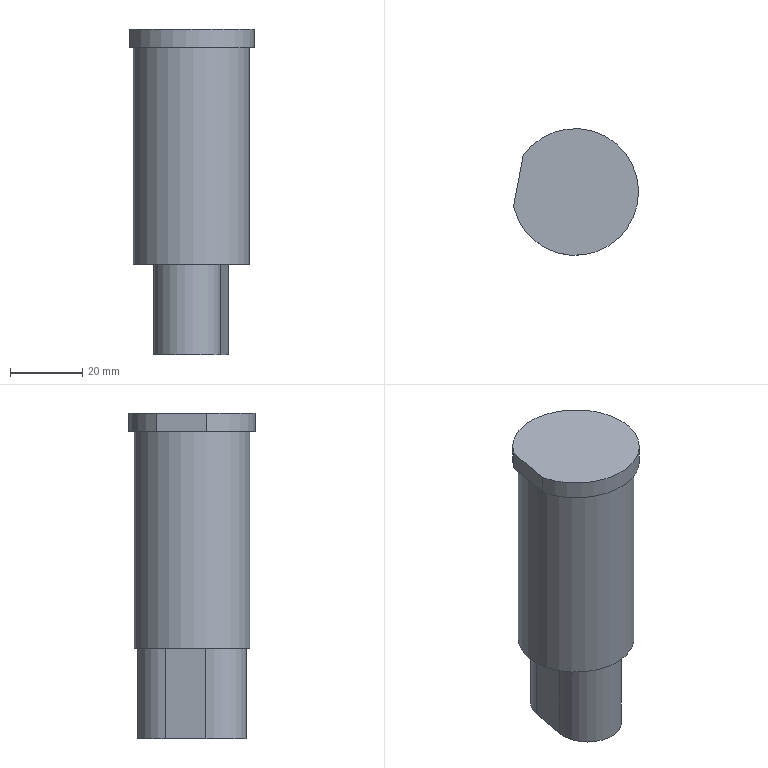Part | NX | features solid 2 | 1 solid | 11 faces | box 34.539 x 35 x 90 mm | volume 65190 mm3 | plane 7 | cylinder 4 | commonest cylinder face diameters 18.7 x2 32 x1 35 x1
STEP:
#1=CARTESIAN_POINT('',(-660.007,435.289,33.));
#2=VERTEX_POINT('',#1);
#3=CARTESIAN_POINT('',(-675.728,438.265,33.));
#4=DIRECTION('',(0.,0.,-1.));
#5=DIRECTION('',(0.9826,-0.186,0.));
#6=AXIS2_PLACEMENT_3D('',#3,#4,#5);
#7=CIRCLE('',#6,16.);
#8=EDGE_CURVE('',#2,#2,#7,.T.);
#9=ORIENTED_EDGE('',*,*,#8,.T.);
#10=EDGE_LOOP('',(#9));
#11=FACE_BOUND('',#10,.T.);
#12=CARTESIAN_POINT('',(-667.602,430.926,33.));
#13=VERTEX_POINT('',#12);
#14=CARTESIAN_POINT('',(-665.481,442.127,33.));
#15=VERTEX_POINT('',#14);
#16=CARTESIAN_POINT('',(-666.541,436.526,33.));
#17=DIRECTION('',(0.186,0.9826,0.));
#18=VECTOR('',#17,1000.);
#19=LINE('',#16,#18);
#20=EDGE_CURVE('',#13,#15,#19,.T.);
#21=ORIENTED_EDGE('',*,*,#20,.T.);
#22=CARTESIAN_POINT('',(-683.855,445.605,33.));
#23=VERTEX_POINT('',#22);
#24=CARTESIAN_POINT('',(-674.668,443.866,33.));
#25=DIRECTION('',(0.,0.,-1.));
#26=DIRECTION('',(0.9826,-0.186,0.));
#27=AXIS2_PLACEMENT_3D('',#24,#25,#26);
#28=CIRCLE('',#27,9.35);
#29=EDGE_CURVE('',#23,#15,#28,.T.);
#30=ORIENTED_EDGE('',*,*,#29,.F.);
#31=CARTESIAN_POINT('',(-685.975,434.403,33.));
#32=VERTEX_POINT('',#31);
#33=CARTESIAN_POINT('',(-684.915,440.004,33.));
#34=DIRECTION('',(0.186,0.9826,0.));
#35=VECTOR('',#34,1000.);
#36=LINE('',#33,#35);
#37=EDGE_CURVE('',#32,#23,#36,.T.);
#38=ORIENTED_EDGE('',*,*,#37,.F.);
#39=CARTESIAN_POINT('',(-676.788,432.665,33.));
#40=DIRECTION('',(0.,0.,-1.));
#41=DIRECTION('',(0.9826,-0.186,0.));
#42=AXIS2_PLACEMENT_3D('',#39,#40,#41);
#43=CIRCLE('',#42,9.35);
#44=EDGE_CURVE('',#13,#32,#43,.T.);
#45=ORIENTED_EDGE('',*,*,#44,.F.);
#46=EDGE_LOOP('',(#21,#30,#38,#45));
#47=FACE_BOUND('',#46,.T.);
#48=CARTESIAN_POINT('',(-675.728,438.265,33.));
#49=DIRECTION('',(0.,0.,1.));
#50=DIRECTION('',(0.9826,-0.186,0.));
#51=AXIS2_PLACEMENT_3D('',#48,#49,#50);
#52=PLANE('',#51);
#53=ADVANCED_FACE('',(#11,#47),#52,.F.);
#54=ORIENTED_EDGE('',*,*,#8,.F.);
#55=EDGE_LOOP('',(#54));
#56=FACE_BOUND('',#55,.T.);
#57=CARTESIAN_POINT('',(-691.449,441.241,93.));
#58=VERTEX_POINT('',#57);
#59=CARTESIAN_POINT('',(-675.728,438.265,93.));
#60=DIRECTION('',(0.,0.,-1.));
#61=DIRECTION('',(0.9826,-0.186,0.));
#62=AXIS2_PLACEMENT_3D('',#59,#60,#61);
#63=CIRCLE('',#62,16.);
#64=EDGE_CURVE('',#58,#58,#63,.T.);
#65=ORIENTED_EDGE('',*,*,#64,.T.);
#66=EDGE_LOOP('',(#65));
#67=FACE_BOUND('',#66,.T.);
#68=CARTESIAN_POINT('',(-675.728,438.265,98.));
#69=DIRECTION('',(0.,0.,-1.));
#70=DIRECTION('',(-0.9826,0.186,0.));
#71=AXIS2_PLACEMENT_3D('',#68,#69,#70);
#72=CYLINDRICAL_SURFACE('',#71,16.);
#73=ADVANCED_FACE('',(#56,#67),#72,.T.);
#74=CARTESIAN_POINT('',(-690.131,448.206,93.));
#75=VERTEX_POINT('',#74);
#76=CARTESIAN_POINT('',(-692.768,434.276,93.));
#77=VERTEX_POINT('',#76);
#78=CARTESIAN_POINT('',(-675.728,438.265,93.));
#79=DIRECTION('',(0.,0.,-1.));
#80=DIRECTION('',(0.9826,-0.186,0.));
#81=AXIS2_PLACEMENT_3D('',#78,#79,#80);
#82=CIRCLE('',#81,17.5);
#83=EDGE_CURVE('',#75,#77,#82,.T.);
#84=ORIENTED_EDGE('',*,*,#83,.T.);
#85=CARTESIAN_POINT('',(-691.449,441.241,93.));
#86=DIRECTION('',(-0.186,-0.9826,0.));
#87=VECTOR('',#86,1000.);
#88=LINE('',#85,#87);
#89=EDGE_CURVE('',#58,#77,#88,.T.);
#90=ORIENTED_EDGE('',*,*,#89,.F.);
#91=ORIENTED_EDGE('',*,*,#64,.F.);
#92=CARTESIAN_POINT('',(-691.449,441.241,93.));
#93=DIRECTION('',(-0.186,-0.9826,0.));
#94=VECTOR('',#93,1000.);
#95=LINE('',#92,#94);
#96=EDGE_CURVE('',#75,#58,#95,.T.);
#97=ORIENTED_EDGE('',*,*,#96,.F.);
#98=EDGE_LOOP('',(#84,#90,#91,#97));
#99=FACE_BOUND('',#98,.T.);
#100=CARTESIAN_POINT('',(-675.728,438.265,93.));
#101=DIRECTION('',(0.,0.,1.));
#102=DIRECTION('',(0.9826,-0.186,0.));
#103=AXIS2_PLACEMENT_3D('',#100,#101,#102);
#104=PLANE('',#103);
#105=ADVANCED_FACE('',(#99),#104,.F.);
#106=CARTESIAN_POINT('',(-692.768,434.276,98.));
#107=VERTEX_POINT('',#106);
#108=CARTESIAN_POINT('',(-692.768,434.276,102.));
#109=DIRECTION('',(0.,0.,-1.));
#110=VECTOR('',#109,1000.);
#111=LINE('',#108,#110);
#112=EDGE_CURVE('',#107,#77,#111,.T.);
#113=ORIENTED_EDGE('',*,*,#112,.T.);
#114=ORIENTED_EDGE('',*,*,#83,.F.);
#115=CARTESIAN_POINT('',(-690.131,448.206,98.));
#116=VERTEX_POINT('',#115);
#117=CARTESIAN_POINT('',(-690.131,448.206,102.));
#118=DIRECTION('',(0.,0.,-1.));
#119=VECTOR('',#118,1000.);
#120=LINE('',#117,#119);
#121=EDGE_CURVE('',#75,#116,#120,.F.);
#122=ORIENTED_EDGE('',*,*,#121,.T.);
#123=CARTESIAN_POINT('',(-675.728,438.265,98.));
#124=DIRECTION('',(0.,0.,-1.));
#125=DIRECTION('',(0.9826,-0.186,0.));
#126=AXIS2_PLACEMENT_3D('',#123,#124,#125);
#127=CIRCLE('',#126,17.5);
#128=EDGE_CURVE('',#116,#107,#127,.T.);
#129=ORIENTED_EDGE('',*,*,#128,.T.);
#130=EDGE_LOOP('',(#113,#114,#122,#129));
#131=FACE_BOUND('',#130,.T.);
#132=CARTESIAN_POINT('',(-675.728,438.265,93.));
#133=DIRECTION('',(0.,0.,1.));
#134=DIRECTION('',(0.9826,-0.186,0.));
#135=AXIS2_PLACEMENT_3D('',#132,#133,#134);
#136=CYLINDRICAL_SURFACE('',#135,17.5);
#137=ADVANCED_FACE('',(#131),#136,.T.);
#138=CARTESIAN_POINT('',(-691.449,441.241,98.));
#139=DIRECTION('',(-0.186,-0.9826,0.));
#140=VECTOR('',#139,1000.);
#141=LINE('',#138,#140);
#142=EDGE_CURVE('',#116,#107,#141,.T.);
#143=ORIENTED_EDGE('',*,*,#142,.T.);
#144=ORIENTED_EDGE('',*,*,#128,.F.);
#145=EDGE_LOOP('',(#143,#144));
#146=FACE_BOUND('',#145,.T.);
#147=CARTESIAN_POINT('',(-675.728,438.265,98.));
#148=DIRECTION('',(0.,0.,1.));
#149=DIRECTION('',(0.9826,-0.186,0.));
#150=AXIS2_PLACEMENT_3D('',#147,#148,#149);
#151=PLANE('',#150);
#152=ADVANCED_FACE('',(#146),#151,.T.);
#153=ORIENTED_EDGE('',*,*,#121,.F.);
#154=ORIENTED_EDGE('',*,*,#96,.T.);
#155=ORIENTED_EDGE('',*,*,#89,.T.);
#156=ORIENTED_EDGE('',*,*,#112,.F.);
#157=ORIENTED_EDGE('',*,*,#142,.F.);
#158=EDGE_LOOP('',(#153,#154,#155,#156,#157));
#159=FACE_BOUND('',#158,.T.);
#160=CARTESIAN_POINT('',(-692.768,434.276,102.));
#161=DIRECTION('',(0.9826,-0.186,0.));
#162=DIRECTION('',(0.,0.,-1.));
#163=AXIS2_PLACEMENT_3D('',#160,#161,#162);
#164=PLANE('',#163);
#165=ADVANCED_FACE('',(#159),#164,.F.);
#166=CARTESIAN_POINT('',(-667.602,430.926,8.));
#167=VERTEX_POINT('',#166);
#168=CARTESIAN_POINT('',(-667.602,430.926,8.));
#169=DIRECTION('',(0.,0.,1.));
#170=VECTOR('',#169,1000.);
#171=LINE('',#168,#170);
#172=EDGE_CURVE('',#167,#13,#171,.T.);
#173=ORIENTED_EDGE('',*,*,#172,.F.);
#174=CARTESIAN_POINT('',(-665.481,442.127,8.));
#175=VERTEX_POINT('',#174);
#176=CARTESIAN_POINT('',(-667.602,430.926,8.));
#177=DIRECTION('',(0.186,0.9826,0.));
#178=VECTOR('',#177,1000.);
#179=LINE('',#176,#178);
#180=EDGE_CURVE('',#167,#175,#179,.T.);
#181=ORIENTED_EDGE('',*,*,#180,.T.);
#182=CARTESIAN_POINT('',(-665.481,442.127,8.));
#183=DIRECTION('',(0.,0.,1.));
#184=VECTOR('',#183,1000.);
#185=LINE('',#182,#184);
#186=EDGE_CURVE('',#175,#15,#185,.T.);
#187=ORIENTED_EDGE('',*,*,#186,.T.);
#188=ORIENTED_EDGE('',*,*,#20,.F.);
#189=EDGE_LOOP('',(#173,#181,#187,#188));
#190=FACE_BOUND('',#189,.T.);
#191=CARTESIAN_POINT('',(-667.602,430.926,8.));
#192=DIRECTION('',(-0.9826,0.186,0.));
#193=DIRECTION('',(0.,0.,1.));
#194=AXIS2_PLACEMENT_3D('',#191,#192,#193);
#195=PLANE('',#194);
#196=ADVANCED_FACE('',(#190),#195,.F.);
#197=ORIENTED_EDGE('',*,*,#29,.T.);
#198=ORIENTED_EDGE('',*,*,#186,.F.);
#199=CARTESIAN_POINT('',(-683.855,445.605,8.));
#200=VERTEX_POINT('',#199);
#201=CARTESIAN_POINT('',(-674.668,443.866,8.));
#202=DIRECTION('',(0.,0.,-1.));
#203=DIRECTION('',(0.9826,-0.186,0.));
#204=AXIS2_PLACEMENT_3D('',#201,#202,#203);
#205=CIRCLE('',#204,9.35);
#206=EDGE_CURVE('',#200,#175,#205,.T.);
#207=ORIENTED_EDGE('',*,*,#206,.F.);
#208=CARTESIAN_POINT('',(-683.855,445.605,8.));
#209=DIRECTION('',(0.,0.,1.));
#210=VECTOR('',#209,1000.);
#211=LINE('',#208,#210);
#212=EDGE_CURVE('',#200,#23,#211,.T.);
#213=ORIENTED_EDGE('',*,*,#212,.T.);
#214=EDGE_LOOP('',(#197,#198,#207,#213));
#215=FACE_BOUND('',#214,.T.);
#216=CARTESIAN_POINT('',(-674.668,443.866,8.));
#217=DIRECTION('',(0.,0.,1.));
#218=DIRECTION('',(0.9826,-0.186,0.));
#219=AXIS2_PLACEMENT_3D('',#216,#217,#218);
#220=CYLINDRICAL_SURFACE('',#219,9.35);
#221=ADVANCED_FACE('',(#215),#220,.T.);
#222=ORIENTED_EDGE('',*,*,#37,.T.);
#223=ORIENTED_EDGE('',*,*,#212,.F.);
#224=CARTESIAN_POINT('',(-685.975,434.403,8.));
#225=VERTEX_POINT('',#224);
#226=CARTESIAN_POINT('',(-685.975,434.403,8.));
#227=DIRECTION('',(0.186,0.9826,0.));
#228=VECTOR('',#227,1000.);
#229=LINE('',#226,#228);
#230=EDGE_CURVE('',#225,#200,#229,.T.);
#231=ORIENTED_EDGE('',*,*,#230,.F.);
#232=CARTESIAN_POINT('',(-685.975,434.403,8.));
#233=DIRECTION('',(0.,0.,1.));
#234=VECTOR('',#233,1000.);
#235=LINE('',#232,#234);
#236=EDGE_CURVE('',#225,#32,#235,.T.);
#237=ORIENTED_EDGE('',*,*,#236,.T.);
#238=EDGE_LOOP('',(#222,#223,#231,#237));
#239=FACE_BOUND('',#238,.T.);
#240=CARTESIAN_POINT('',(-685.975,434.403,8.));
#241=DIRECTION('',(-0.9826,0.186,0.));
#242=DIRECTION('',(0.,0.,1.));
#243=AXIS2_PLACEMENT_3D('',#240,#241,#242);
#244=PLANE('',#243);
#245=ADVANCED_FACE('',(#239),#244,.T.);
#246=ORIENTED_EDGE('',*,*,#44,.T.);
#247=ORIENTED_EDGE('',*,*,#236,.F.);
#248=CARTESIAN_POINT('',(-676.788,432.665,8.));
#249=DIRECTION('',(0.,0.,-1.));
#250=DIRECTION('',(0.9826,-0.186,0.));
#251=AXIS2_PLACEMENT_3D('',#248,#249,#250);
#252=CIRCLE('',#251,9.35);
#253=EDGE_CURVE('',#167,#225,#252,.T.);
#254=ORIENTED_EDGE('',*,*,#253,.F.);
#255=ORIENTED_EDGE('',*,*,#172,.T.);
#256=EDGE_LOOP('',(#246,#247,#254,#255));
#257=FACE_BOUND('',#256,.T.);
#258=CARTESIAN_POINT('',(-676.788,432.665,8.));
#259=DIRECTION('',(0.,0.,1.));
#260=DIRECTION('',(0.9826,-0.186,0.));
#261=AXIS2_PLACEMENT_3D('',#258,#259,#260);
#262=CYLINDRICAL_SURFACE('',#261,9.35);
#263=ADVANCED_FACE('',(#257),#262,.T.);
#264=ORIENTED_EDGE('',*,*,#180,.F.);
#265=ORIENTED_EDGE('',*,*,#253,.T.);
#266=ORIENTED_EDGE('',*,*,#230,.T.);
#267=ORIENTED_EDGE('',*,*,#206,.T.);
#268=EDGE_LOOP('',(#264,#265,#266,#267));
#269=FACE_BOUND('',#268,.T.);
#270=CARTESIAN_POINT('',(-674.668,443.866,8.));
#271=DIRECTION('',(0.,0.,1.));
#272=DIRECTION('',(0.9826,-0.186,0.));
#273=AXIS2_PLACEMENT_3D('',#270,#271,#272);
#274=PLANE('',#273);
#275=ADVANCED_FACE('',(#269),#274,.F.);
#276=CLOSED_SHELL('',(#53,#73,#105,#137,#152,#165,#196,#221,#245,#263,#275));
#277=MANIFOLD_SOLID_BREP('',#276);
#278=(LENGTH_UNIT()NAMED_UNIT(*)SI_UNIT(.MILLI.,.METRE.));
#279=UNCERTAINTY_MEASURE_WITH_UNIT(LENGTH_MEASURE(0.00001),#278,'','');
#280=(NAMED_UNIT(*)PLANE_ANGLE_UNIT()SI_UNIT($,.RADIAN.));
#281=(NAMED_UNIT(*)SI_UNIT($,.STERADIAN.)SOLID_ANGLE_UNIT());
#282=(GEOMETRIC_REPRESENTATION_CONTEXT(3)GLOBAL_UNCERTAINTY_ASSIGNED_CONTEXT((#279))GLOBAL_UNIT_ASSIGNED_CONTEXT((#278,#280,#281))REPRESENTATION_CONTEXT('',''));
#283=ADVANCED_BREP_SHAPE_REPRESENTATION('',(#277),#282);